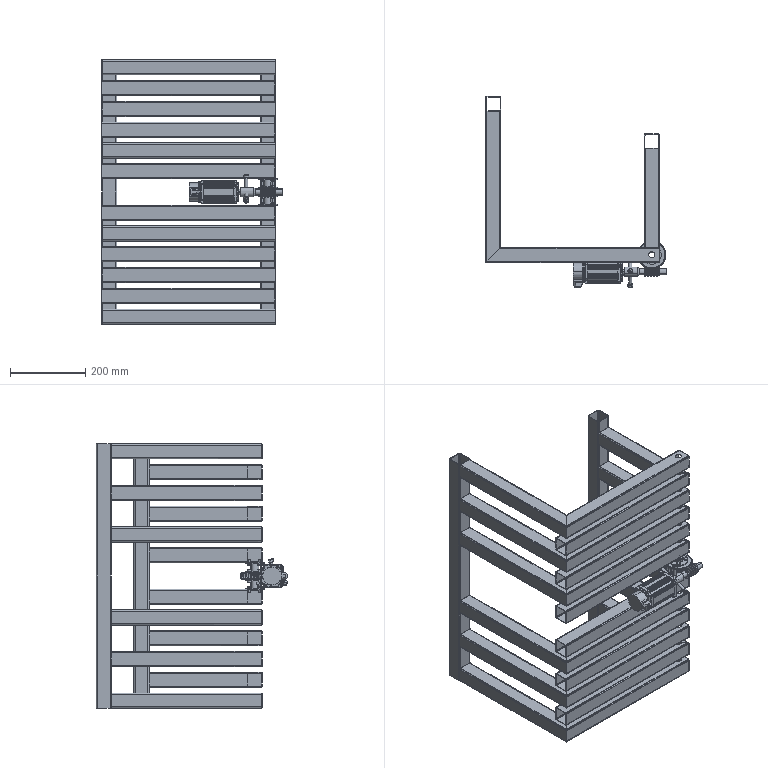Part | SolidWorks | features ReferencePattern 17, LocalCirPattern 2, MirrorCompFeat 1 | 50 solids | 2410 faces | box 477.948 x 507.594 x 700 mm | volume 2896175 mm3 | plane 979 | cylinder 833 | cone 239 | torus 197 | spline 110 | sphere 52 | commonest cylinder face diameters 0.4 x216 6 x168 3 x124 16 x64 73.955 x55 4.2 x28